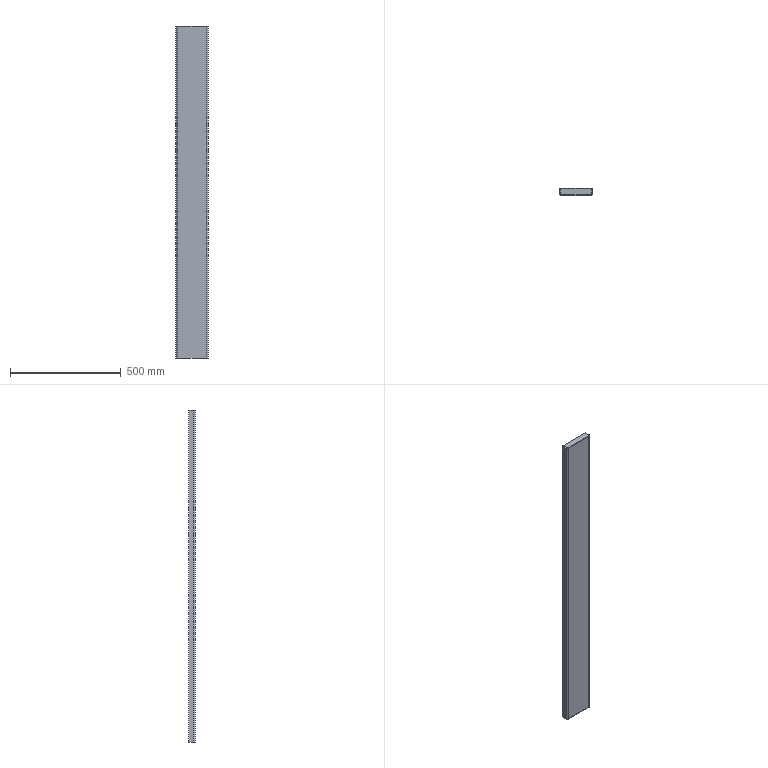Part | SolidWorks | features ICE 2, Extrusion 1 | 3 solids | 30 faces | box 145 x 30 x 1500 mm | volume 892760 mm3 | plane 26 | cylinder 4 | commonest cylinder face diameters 10 x2 16 x2
STEP:
#1=CARTESIAN_POINT('',(145.,-22.,0.));
#2=VERTEX_POINT('',#1);
#3=CARTESIAN_POINT('',(145.,0.,0.));
#4=VERTEX_POINT('',#3);
#5=CARTESIAN_POINT('',(145.,-22.,0.));
#6=DIRECTION('',(0.,1.,0.));
#7=VECTOR('',#6,1000.);
#8=LINE('',#5,#7);
#9=EDGE_CURVE('',#2,#4,#8,.T.);
#10=ORIENTED_EDGE('',*,*,#9,.T.);
#11=CARTESIAN_POINT('',(145.,0.,1500.));
#12=VERTEX_POINT('',#11);
#13=CARTESIAN_POINT('',(145.,0.,1500.));
#14=DIRECTION('',(0.,0.,-1.));
#15=VECTOR('',#14,1000.);
#16=LINE('',#13,#15);
#17=EDGE_CURVE('',#12,#4,#16,.T.);
#18=ORIENTED_EDGE('',*,*,#17,.F.);
#19=CARTESIAN_POINT('',(145.,-22.,1500.));
#20=VERTEX_POINT('',#19);
#21=CARTESIAN_POINT('',(145.,-22.,1500.));
#22=DIRECTION('',(0.,1.,0.));
#23=VECTOR('',#22,1000.);
#24=LINE('',#21,#23);
#25=EDGE_CURVE('',#20,#12,#24,.T.);
#26=ORIENTED_EDGE('',*,*,#25,.F.);
#27=CARTESIAN_POINT('',(145.,-22.,1500.));
#28=DIRECTION('',(0.,0.,-1.));
#29=VECTOR('',#28,1000.);
#30=LINE('',#27,#29);
#31=EDGE_CURVE('',#20,#2,#30,.T.);
#32=ORIENTED_EDGE('',*,*,#31,.T.);
#33=EDGE_LOOP('',(#10,#18,#26,#32));
#34=FACE_OUTER_BOUND('',#33,.T.);
#35=CARTESIAN_POINT('',(145.,-22.,1500.));
#36=DIRECTION('',(-1.,0.,0.));
#37=DIRECTION('',(0.,0.,1.));
#38=AXIS2_PLACEMENT_3D('',#35,#36,#37);
#39=PLANE('',#38);
#40=ADVANCED_FACE('',(#34),#39,.F.);
#41=CARTESIAN_POINT('',(142.,0.,0.));
#42=VERTEX_POINT('',#41);
#43=CARTESIAN_POINT('',(145.,0.,0.));
#44=DIRECTION('',(-1.,0.,0.));
#45=VECTOR('',#44,1000.);
#46=LINE('',#43,#45);
#47=EDGE_CURVE('',#4,#42,#46,.T.);
#48=ORIENTED_EDGE('',*,*,#47,.T.);
#49=CARTESIAN_POINT('',(142.,0.,1500.));
#50=VERTEX_POINT('',#49);
#51=CARTESIAN_POINT('',(142.,0.,1500.));
#52=DIRECTION('',(0.,0.,-1.));
#53=VECTOR('',#52,1000.);
#54=LINE('',#51,#53);
#55=EDGE_CURVE('',#50,#42,#54,.T.);
#56=ORIENTED_EDGE('',*,*,#55,.F.);
#57=CARTESIAN_POINT('',(145.,0.,1500.));
#58=DIRECTION('',(-1.,0.,0.));
#59=VECTOR('',#58,1000.);
#60=LINE('',#57,#59);
#61=EDGE_CURVE('',#12,#50,#60,.T.);
#62=ORIENTED_EDGE('',*,*,#61,.F.);
#63=ORIENTED_EDGE('',*,*,#17,.T.);
#64=EDGE_LOOP('',(#48,#56,#62,#63));
#65=FACE_OUTER_BOUND('',#64,.T.);
#66=CARTESIAN_POINT('',(145.,0.,1500.));
#67=DIRECTION('',(0.,-1.,0.));
#68=DIRECTION('',(0.,0.,-1.));
#69=AXIS2_PLACEMENT_3D('',#66,#67,#68);
#70=PLANE('',#69);
#71=ADVANCED_FACE('',(#65),#70,.F.);
#72=CARTESIAN_POINT('',(142.,-22.,0.));
#73=VERTEX_POINT('',#72);
#74=CARTESIAN_POINT('',(142.,-22.,0.));
#75=DIRECTION('',(0.,1.,0.));
#76=VECTOR('',#75,1000.);
#77=LINE('',#74,#76);
#78=EDGE_CURVE('',#73,#42,#77,.T.);
#79=ORIENTED_EDGE('',*,*,#78,.F.);
#80=CARTESIAN_POINT('',(142.,-22.,1500.));
#81=VERTEX_POINT('',#80);
#82=CARTESIAN_POINT('',(142.,-22.,1500.));
#83=DIRECTION('',(0.,0.,-1.));
#84=VECTOR('',#83,1000.);
#85=LINE('',#82,#84);
#86=EDGE_CURVE('',#81,#73,#85,.T.);
#87=ORIENTED_EDGE('',*,*,#86,.F.);
#88=CARTESIAN_POINT('',(142.,-22.,1500.));
#89=DIRECTION('',(0.,1.,0.));
#90=VECTOR('',#89,1000.);
#91=LINE('',#88,#90);
#92=EDGE_CURVE('',#81,#50,#91,.T.);
#93=ORIENTED_EDGE('',*,*,#92,.T.);
#94=ORIENTED_EDGE('',*,*,#55,.T.);
#95=EDGE_LOOP('',(#79,#87,#93,#94));
#96=FACE_OUTER_BOUND('',#95,.T.);
#97=CARTESIAN_POINT('',(142.,-22.,1500.));
#98=DIRECTION('',(-1.,0.,0.));
#99=DIRECTION('',(0.,0.,1.));
#100=AXIS2_PLACEMENT_3D('',#97,#98,#99);
#101=PLANE('',#100);
#102=ADVANCED_FACE('',(#96),#101,.T.);
#103=CARTESIAN_POINT('',(137.,-27.,0.));
#104=VERTEX_POINT('',#103);
#105=CARTESIAN_POINT('',(137.,-22.,0.));
#106=DIRECTION('',(0.,0.,1.));
#107=DIRECTION('',(1.,0.,0.));
#108=AXIS2_PLACEMENT_3D('',#105,#106,#107);
#109=CIRCLE('',#108,5.);
#110=EDGE_CURVE('',#104,#73,#109,.T.);
#111=ORIENTED_EDGE('',*,*,#110,.F.);
#112=CARTESIAN_POINT('',(137.,-27.,1500.));
#113=VERTEX_POINT('',#112);
#114=CARTESIAN_POINT('',(137.,-27.,1500.));
#115=DIRECTION('',(0.,0.,-1.));
#116=VECTOR('',#115,1000.);
#117=LINE('',#114,#116);
#118=EDGE_CURVE('',#113,#104,#117,.T.);
#119=ORIENTED_EDGE('',*,*,#118,.F.);
#120=CARTESIAN_POINT('',(137.,-22.,1500.));
#121=DIRECTION('',(0.,0.,1.));
#122=DIRECTION('',(1.,0.,0.));
#123=AXIS2_PLACEMENT_3D('',#120,#121,#122);
#124=CIRCLE('',#123,5.);
#125=EDGE_CURVE('',#113,#81,#124,.T.);
#126=ORIENTED_EDGE('',*,*,#125,.T.);
#127=ORIENTED_EDGE('',*,*,#86,.T.);
#128=EDGE_LOOP('',(#111,#119,#126,#127));
#129=FACE_OUTER_BOUND('',#128,.T.);
#130=CARTESIAN_POINT('',(137.,-22.,1500.));
#131=DIRECTION('',(0.,0.,-1.));
#132=DIRECTION('',(-1.,0.,0.));
#133=AXIS2_PLACEMENT_3D('',#130,#131,#132);
#134=CYLINDRICAL_SURFACE('',#133,5.);
#135=ADVANCED_FACE('',(#129),#134,.F.);
#136=CARTESIAN_POINT('',(8.,-27.,0.));
#137=VERTEX_POINT('',#136);
#138=CARTESIAN_POINT('',(8.,-27.,0.));
#139=DIRECTION('',(1.,0.,0.));
#140=VECTOR('',#139,1000.);
#141=LINE('',#138,#140);
#142=EDGE_CURVE('',#137,#104,#141,.T.);
#143=ORIENTED_EDGE('',*,*,#142,.F.);
#144=CARTESIAN_POINT('',(8.,-27.,1500.));
#145=VERTEX_POINT('',#144);
#146=CARTESIAN_POINT('',(8.,-27.,1500.));
#147=DIRECTION('',(0.,0.,-1.));
#148=VECTOR('',#147,1000.);
#149=LINE('',#146,#148);
#150=EDGE_CURVE('',#145,#137,#149,.T.);
#151=ORIENTED_EDGE('',*,*,#150,.F.);
#152=CARTESIAN_POINT('',(8.,-27.,1500.));
#153=DIRECTION('',(1.,0.,0.));
#154=VECTOR('',#153,1000.);
#155=LINE('',#152,#154);
#156=EDGE_CURVE('',#145,#113,#155,.T.);
#157=ORIENTED_EDGE('',*,*,#156,.T.);
#158=ORIENTED_EDGE('',*,*,#118,.T.);
#159=EDGE_LOOP('',(#143,#151,#157,#158));
#160=FACE_OUTER_BOUND('',#159,.T.);
#161=CARTESIAN_POINT('',(8.,-27.,1500.));
#162=DIRECTION('',(0.,1.,0.));
#163=DIRECTION('',(0.,0.,1.));
#164=AXIS2_PLACEMENT_3D('',#161,#162,#163);
#165=PLANE('',#164);
#166=ADVANCED_FACE('',(#160),#165,.T.);
#167=CARTESIAN_POINT('',(3.,-22.,0.));
#168=VERTEX_POINT('',#167);
#169=CARTESIAN_POINT('',(8.,-22.,0.));
#170=DIRECTION('',(0.,0.,1.));
#171=DIRECTION('',(1.,0.,0.));
#172=AXIS2_PLACEMENT_3D('',#169,#170,#171);
#173=CIRCLE('',#172,5.);
#174=EDGE_CURVE('',#168,#137,#173,.T.);
#175=ORIENTED_EDGE('',*,*,#174,.F.);
#176=CARTESIAN_POINT('',(3.,-22.,1500.));
#177=VERTEX_POINT('',#176);
#178=CARTESIAN_POINT('',(3.,-22.,1500.));
#179=DIRECTION('',(0.,0.,-1.));
#180=VECTOR('',#179,1000.);
#181=LINE('',#178,#180);
#182=EDGE_CURVE('',#177,#168,#181,.T.);
#183=ORIENTED_EDGE('',*,*,#182,.F.);
#184=CARTESIAN_POINT('',(8.,-22.,1500.));
#185=DIRECTION('',(0.,0.,1.));
#186=DIRECTION('',(1.,0.,0.));
#187=AXIS2_PLACEMENT_3D('',#184,#185,#186);
#188=CIRCLE('',#187,5.);
#189=EDGE_CURVE('',#177,#145,#188,.T.);
#190=ORIENTED_EDGE('',*,*,#189,.T.);
#191=ORIENTED_EDGE('',*,*,#150,.T.);
#192=EDGE_LOOP('',(#175,#183,#190,#191));
#193=FACE_OUTER_BOUND('',#192,.T.);
#194=CARTESIAN_POINT('',(8.,-22.,1500.));
#195=DIRECTION('',(0.,0.,-1.));
#196=DIRECTION('',(-1.,0.,0.));
#197=AXIS2_PLACEMENT_3D('',#194,#195,#196);
#198=CYLINDRICAL_SURFACE('',#197,5.);
#199=ADVANCED_FACE('',(#193),#198,.F.);
#200=CARTESIAN_POINT('',(3.,0.,0.));
#201=VERTEX_POINT('',#200);
#202=CARTESIAN_POINT('',(3.,0.,0.));
#203=DIRECTION('',(0.,-1.,0.));
#204=VECTOR('',#203,1000.);
#205=LINE('',#202,#204);
#206=EDGE_CURVE('',#201,#168,#205,.T.);
#207=ORIENTED_EDGE('',*,*,#206,.F.);
#208=CARTESIAN_POINT('',(3.,0.,1500.));
#209=VERTEX_POINT('',#208);
#210=CARTESIAN_POINT('',(3.,0.,1500.));
#211=DIRECTION('',(0.,0.,-1.));
#212=VECTOR('',#211,1000.);
#213=LINE('',#210,#212);
#214=EDGE_CURVE('',#209,#201,#213,.T.);
#215=ORIENTED_EDGE('',*,*,#214,.F.);
#216=CARTESIAN_POINT('',(3.,0.,1500.));
#217=DIRECTION('',(0.,-1.,0.));
#218=VECTOR('',#217,1000.);
#219=LINE('',#216,#218);
#220=EDGE_CURVE('',#209,#177,#219,.T.);
#221=ORIENTED_EDGE('',*,*,#220,.T.);
#222=ORIENTED_EDGE('',*,*,#182,.T.);
#223=EDGE_LOOP('',(#207,#215,#221,#222));
#224=FACE_OUTER_BOUND('',#223,.T.);
#225=CARTESIAN_POINT('',(3.,0.,1500.));
#226=DIRECTION('',(1.,0.,0.));
#227=DIRECTION('',(0.,0.,-1.));
#228=AXIS2_PLACEMENT_3D('',#225,#226,#227);
#229=PLANE('',#228);
#230=ADVANCED_FACE('',(#224),#229,.T.);
#231=CARTESIAN_POINT('',(0.,0.,0.));
#232=VERTEX_POINT('',#231);
#233=CARTESIAN_POINT('',(0.,0.,0.));
#234=DIRECTION('',(1.,0.,0.));
#235=VECTOR('',#234,1000.);
#236=LINE('',#233,#235);
#237=EDGE_CURVE('',#232,#201,#236,.T.);
#238=ORIENTED_EDGE('',*,*,#237,.F.);
#239=CARTESIAN_POINT('',(0.,0.,1500.));
#240=VERTEX_POINT('',#239);
#241=CARTESIAN_POINT('',(0.,0.,1500.));
#242=DIRECTION('',(0.,0.,-1.));
#243=VECTOR('',#242,1000.);
#244=LINE('',#241,#243);
#245=EDGE_CURVE('',#240,#232,#244,.T.);
#246=ORIENTED_EDGE('',*,*,#245,.F.);
#247=CARTESIAN_POINT('',(0.,0.,1500.));
#248=DIRECTION('',(1.,0.,0.));
#249=VECTOR('',#248,1000.);
#250=LINE('',#247,#249);
#251=EDGE_CURVE('',#240,#209,#250,.T.);
#252=ORIENTED_EDGE('',*,*,#251,.T.);
#253=ORIENTED_EDGE('',*,*,#214,.T.);
#254=EDGE_LOOP('',(#238,#246,#252,#253));
#255=FACE_OUTER_BOUND('',#254,.T.);
#256=CARTESIAN_POINT('',(0.,0.,1500.));
#257=DIRECTION('',(0.,1.,0.));
#258=DIRECTION('',(0.,0.,1.));
#259=AXIS2_PLACEMENT_3D('',#256,#257,#258);
#260=PLANE('',#259);
#261=ADVANCED_FACE('',(#255),#260,.T.);
#262=CARTESIAN_POINT('',(0.,-22.,0.));
#263=VERTEX_POINT('',#262);
#264=CARTESIAN_POINT('',(0.,0.,0.));
#265=DIRECTION('',(0.,-1.,0.));
#266=VECTOR('',#265,1000.);
#267=LINE('',#264,#266);
#268=EDGE_CURVE('',#232,#263,#267,.T.);
#269=ORIENTED_EDGE('',*,*,#268,.T.);
#270=CARTESIAN_POINT('',(0.,-22.,1500.));
#271=VERTEX_POINT('',#270);
#272=CARTESIAN_POINT('',(0.,-22.,1500.));
#273=DIRECTION('',(0.,0.,-1.));
#274=VECTOR('',#273,1000.);
#275=LINE('',#272,#274);
#276=EDGE_CURVE('',#271,#263,#275,.T.);
#277=ORIENTED_EDGE('',*,*,#276,.F.);
#278=CARTESIAN_POINT('',(0.,0.,1500.));
#279=DIRECTION('',(0.,-1.,0.));
#280=VECTOR('',#279,1000.);
#281=LINE('',#278,#280);
#282=EDGE_CURVE('',#240,#271,#281,.T.);
#283=ORIENTED_EDGE('',*,*,#282,.F.);
#284=ORIENTED_EDGE('',*,*,#245,.T.);
#285=EDGE_LOOP('',(#269,#277,#283,#284));
#286=FACE_OUTER_BOUND('',#285,.T.);
#287=CARTESIAN_POINT('',(0.,0.,1500.));
#288=DIRECTION('',(1.,0.,0.));
#289=DIRECTION('',(0.,0.,-1.));
#290=AXIS2_PLACEMENT_3D('',#287,#288,#289);
#291=PLANE('',#290);
#292=ADVANCED_FACE('',(#286),#291,.F.);
#293=CARTESIAN_POINT('',(8.,-30.,0.));
#294=VERTEX_POINT('',#293);
#295=CARTESIAN_POINT('',(8.,-22.,0.));
#296=DIRECTION('',(0.,0.,1.));
#297=DIRECTION('',(1.,0.,0.));
#298=AXIS2_PLACEMENT_3D('',#295,#296,#297);
#299=CIRCLE('',#298,8.);
#300=EDGE_CURVE('',#263,#294,#299,.T.);
#301=ORIENTED_EDGE('',*,*,#300,.T.);
#302=CARTESIAN_POINT('',(8.,-30.,1500.));
#303=VERTEX_POINT('',#302);
#304=CARTESIAN_POINT('',(8.,-30.,1500.));
#305=DIRECTION('',(0.,0.,-1.));
#306=VECTOR('',#305,1000.);
#307=LINE('',#304,#306);
#308=EDGE_CURVE('',#303,#294,#307,.T.);
#309=ORIENTED_EDGE('',*,*,#308,.F.);
#310=CARTESIAN_POINT('',(8.,-22.,1500.));
#311=DIRECTION('',(0.,0.,1.));
#312=DIRECTION('',(1.,0.,0.));
#313=AXIS2_PLACEMENT_3D('',#310,#311,#312);
#314=CIRCLE('',#313,8.);
#315=EDGE_CURVE('',#271,#303,#314,.T.);
#316=ORIENTED_EDGE('',*,*,#315,.F.);
#317=ORIENTED_EDGE('',*,*,#276,.T.);
#318=EDGE_LOOP('',(#301,#309,#316,#317));
#319=FACE_OUTER_BOUND('',#318,.T.);
#320=CARTESIAN_POINT('',(8.,-22.,1500.));
#321=DIRECTION('',(0.,0.,-1.));
#322=DIRECTION('',(-1.,0.,0.));
#323=AXIS2_PLACEMENT_3D('',#320,#321,#322);
#324=CYLINDRICAL_SURFACE('',#323,8.);
#325=ADVANCED_FACE('',(#319),#324,.T.);
#326=CARTESIAN_POINT('',(137.,-30.,0.));
#327=VERTEX_POINT('',#326);
#328=CARTESIAN_POINT('',(8.,-30.,0.));
#329=DIRECTION('',(1.,0.,0.));
#330=VECTOR('',#329,1000.);
#331=LINE('',#328,#330);
#332=EDGE_CURVE('',#294,#327,#331,.T.);
#333=ORIENTED_EDGE('',*,*,#332,.T.);
#334=CARTESIAN_POINT('',(137.,-30.,1500.));
#335=VERTEX_POINT('',#334);
#336=CARTESIAN_POINT('',(137.,-30.,1500.));
#337=DIRECTION('',(0.,0.,-1.));
#338=VECTOR('',#337,1000.);
#339=LINE('',#336,#338);
#340=EDGE_CURVE('',#335,#327,#339,.T.);
#341=ORIENTED_EDGE('',*,*,#340,.F.);
#342=CARTESIAN_POINT('',(8.,-30.,1500.));
#343=DIRECTION('',(1.,0.,0.));
#344=VECTOR('',#343,1000.);
#345=LINE('',#342,#344);
#346=EDGE_CURVE('',#303,#335,#345,.T.);
#347=ORIENTED_EDGE('',*,*,#346,.F.);
#348=ORIENTED_EDGE('',*,*,#308,.T.);
#349=EDGE_LOOP('',(#333,#341,#347,#348));
#350=FACE_OUTER_BOUND('',#349,.T.);
#351=CARTESIAN_POINT('',(8.,-30.,1500.));
#352=DIRECTION('',(0.,1.,0.));
#353=DIRECTION('',(0.,0.,1.));
#354=AXIS2_PLACEMENT_3D('',#351,#352,#353);
#355=PLANE('',#354);
#356=ADVANCED_FACE('',(#350),#355,.F.);
#357=CARTESIAN_POINT('',(137.,-22.,0.));
#358=DIRECTION('',(0.,0.,1.));
#359=DIRECTION('',(1.,0.,0.));
#360=AXIS2_PLACEMENT_3D('',#357,#358,#359);
#361=CIRCLE('',#360,8.);
#362=EDGE_CURVE('',#327,#2,#361,.T.);
#363=ORIENTED_EDGE('',*,*,#362,.T.);
#364=ORIENTED_EDGE('',*,*,#31,.F.);
#365=CARTESIAN_POINT('',(137.,-22.,1500.));
#366=DIRECTION('',(0.,0.,1.));
#367=DIRECTION('',(1.,0.,0.));
#368=AXIS2_PLACEMENT_3D('',#365,#366,#367);
#369=CIRCLE('',#368,8.);
#370=EDGE_CURVE('',#335,#20,#369,.T.);
#371=ORIENTED_EDGE('',*,*,#370,.F.);
#372=ORIENTED_EDGE('',*,*,#340,.T.);
#373=EDGE_LOOP('',(#363,#364,#371,#372));
#374=FACE_OUTER_BOUND('',#373,.T.);
#375=CARTESIAN_POINT('',(137.,-22.,1500.));
#376=DIRECTION('',(0.,0.,-1.));
#377=DIRECTION('',(-1.,0.,0.));
#378=AXIS2_PLACEMENT_3D('',#375,#376,#377);
#379=CYLINDRICAL_SURFACE('',#378,8.);
#380=ADVANCED_FACE('',(#374),#379,.T.);
#381=ORIENTED_EDGE('',*,*,#25,.T.);
#382=ORIENTED_EDGE('',*,*,#61,.T.);
#383=ORIENTED_EDGE('',*,*,#92,.F.);
#384=ORIENTED_EDGE('',*,*,#125,.F.);
#385=ORIENTED_EDGE('',*,*,#156,.F.);
#386=ORIENTED_EDGE('',*,*,#189,.F.);
#387=ORIENTED_EDGE('',*,*,#220,.F.);
#388=ORIENTED_EDGE('',*,*,#251,.F.);
#389=ORIENTED_EDGE('',*,*,#282,.T.);
#390=ORIENTED_EDGE('',*,*,#315,.T.);
#391=ORIENTED_EDGE('',*,*,#346,.T.);
#392=ORIENTED_EDGE('',*,*,#370,.T.);
#393=EDGE_LOOP('',(#381,#382,#383,#384,#385,#386,#387,#388,#389,#390,#391,#392));
#394=FACE_OUTER_BOUND('',#393,.T.);
#395=CARTESIAN_POINT('',(137.,-22.,1500.));
#396=DIRECTION('',(0.,0.,1.));
#397=DIRECTION('',(1.,0.,0.));
#398=AXIS2_PLACEMENT_3D('',#395,#396,#397);
#399=PLANE('',#398);
#400=ADVANCED_FACE('',(#394),#399,.T.);
#401=ORIENTED_EDGE('',*,*,#9,.F.);
#402=ORIENTED_EDGE('',*,*,#362,.F.);
#403=ORIENTED_EDGE('',*,*,#332,.F.);
#404=ORIENTED_EDGE('',*,*,#300,.F.);
#405=ORIENTED_EDGE('',*,*,#268,.F.);
#406=ORIENTED_EDGE('',*,*,#237,.T.);
#407=ORIENTED_EDGE('',*,*,#206,.T.);
#408=ORIENTED_EDGE('',*,*,#174,.T.);
#409=ORIENTED_EDGE('',*,*,#142,.T.);
#410=ORIENTED_EDGE('',*,*,#110,.T.);
#411=ORIENTED_EDGE('',*,*,#78,.T.);
#412=ORIENTED_EDGE('',*,*,#47,.F.);
#413=EDGE_LOOP('',(#401,#402,#403,#404,#405,#406,#407,#408,#409,#410,#411,#412));
#414=FACE_OUTER_BOUND('',#413,.T.);
#415=CARTESIAN_POINT('',(137.,-22.,0.));
#416=DIRECTION('',(0.,0.,1.));
#417=DIRECTION('',(1.,0.,0.));
#418=AXIS2_PLACEMENT_3D('',#415,#416,#417);
#419=PLANE('',#418);
#420=ADVANCED_FACE('',(#414),#419,.F.);
#421=CLOSED_SHELL('',(#40,#71,#102,#135,#166,#199,#230,#261,#292,#325,#356,#380,#400,#420));
#422=MANIFOLD_SOLID_BREP('',#421);
#423=CARTESIAN_POINT('',(8.,-27.,1500.));
#424=VERTEX_POINT('',#423);
#425=CARTESIAN_POINT('',(3.,-22.,1500.));
#426=VERTEX_POINT('',#425);
#427=CARTESIAN_POINT('',(8.,-27.,1500.));
#428=DIRECTION('',(-0.7071,0.7071,0.));
#429=VECTOR('',#428,1000.);
#430=LINE('',#427,#429);
#431=EDGE_CURVE('',#424,#426,#430,.T.);
#432=ORIENTED_EDGE('',*,*,#431,.T.);
#433=CARTESIAN_POINT('',(3.,-22.,1497.));
#434=VERTEX_POINT('',#433);
#435=CARTESIAN_POINT('',(3.,-22.,1497.));
#436=DIRECTION('',(0.,0.,1.));
#437=VECTOR('',#436,1000.);
#438=LINE('',#435,#437);
#439=EDGE_CURVE('',#434,#426,#438,.T.);
#440=ORIENTED_EDGE('',*,*,#439,.F.);
#441=CARTESIAN_POINT('',(8.,-27.,1497.));
#442=VERTEX_POINT('',#441);
#443=CARTESIAN_POINT('',(8.,-27.,1497.));
#444=DIRECTION('',(-0.7071,0.7071,0.));
#445=VECTOR('',#444,1000.);
#446=LINE('',#443,#445);
#447=EDGE_CURVE('',#442,#434,#446,.T.);
#448=ORIENTED_EDGE('',*,*,#447,.F.);
#449=CARTESIAN_POINT('',(8.,-27.,1497.));
#450=DIRECTION('',(0.,0.,1.));
#451=VECTOR('',#450,1000.);
#452=LINE('',#449,#451);
#453=EDGE_CURVE('',#442,#424,#452,.T.);
#454=ORIENTED_EDGE('',*,*,#453,.T.);
#455=EDGE_LOOP('',(#432,#440,#448,#454));
#456=FACE_OUTER_BOUND('',#455,.T.);
#457=CARTESIAN_POINT('',(8.,-27.,1497.));
#458=DIRECTION('',(0.7071,0.7071,0.));
#459=DIRECTION('',(-0.7071,0.7071,0.));
#460=AXIS2_PLACEMENT_3D('',#457,#458,#459);
#461=PLANE('',#460);
#462=ADVANCED_FACE('',(#456),#461,.F.);
#463=CARTESIAN_POINT('',(3.,0.,1500.));
#464=VERTEX_POINT('',#463);
#465=CARTESIAN_POINT('',(3.,-22.,1500.));
#466=DIRECTION('',(0.,1.,0.));
#467=VECTOR('',#466,1000.);
#468=LINE('',#465,#467);
#469=EDGE_CURVE('',#426,#464,#468,.T.);
#470=ORIENTED_EDGE('',*,*,#469,.T.);
#471=CARTESIAN_POINT('',(3.,0.,1497.));
#472=VERTEX_POINT('',#471);
#473=CARTESIAN_POINT('',(3.,0.,1497.));
#474=DIRECTION('',(0.,0.,1.));
#475=VECTOR('',#474,1000.);
#476=LINE('',#473,#475);
#477=EDGE_CURVE('',#472,#464,#476,.T.);
#478=ORIENTED_EDGE('',*,*,#477,.F.);
#479=CARTESIAN_POINT('',(3.,-22.,1497.));
#480=DIRECTION('',(0.,1.,0.));
#481=VECTOR('',#480,1000.);
#482=LINE('',#479,#481);
#483=EDGE_CURVE('',#434,#472,#482,.T.);
#484=ORIENTED_EDGE('',*,*,#483,.F.);
#485=ORIENTED_EDGE('',*,*,#439,.T.);
#486=EDGE_LOOP('',(#470,#478,#484,#485));
#487=FACE_OUTER_BOUND('',#486,.T.);
#488=CARTESIAN_POINT('',(3.,-22.,1497.));
#489=DIRECTION('',(1.,0.,0.));
#490=DIRECTION('',(0.,1.,0.));
#491=AXIS2_PLACEMENT_3D('',#488,#489,#490);
#492=PLANE('',#491);
#493=ADVANCED_FACE('',(#487),#492,.F.);
#494=CARTESIAN_POINT('',(142.,0.,1500.));
#495=VERTEX_POINT('',#494);
#496=CARTESIAN_POINT('',(3.,0.,1500.));
#497=DIRECTION('',(1.,0.,0.));
#498=VECTOR('',#497,1000.);
#499=LINE('',#496,#498);
#500=EDGE_CURVE('',#464,#495,#499,.T.);
#501=ORIENTED_EDGE('',*,*,#500,.T.);
#502=CARTESIAN_POINT('',(142.,0.,1497.));
#503=VERTEX_POINT('',#502);
#504=CARTESIAN_POINT('',(142.,0.,1497.));
#505=DIRECTION('',(0.,0.,1.));
#506=VECTOR('',#505,1000.);
#507=LINE('',#504,#506);
#508=EDGE_CURVE('',#503,#495,#507,.T.);
#509=ORIENTED_EDGE('',*,*,#508,.F.);
#510=CARTESIAN_POINT('',(3.,0.,1497.));
#511=DIRECTION('',(1.,0.,0.));
#512=VECTOR('',#511,1000.);
#513=LINE('',#510,#512);
#514=EDGE_CURVE('',#472,#503,#513,.T.);
#515=ORIENTED_EDGE('',*,*,#514,.F.);
#516=ORIENTED_EDGE('',*,*,#477,.T.);
#517=EDGE_LOOP('',(#501,#509,#515,#516));
#518=FACE_OUTER_BOUND('',#517,.T.);
#519=CARTESIAN_POINT('',(3.,0.,1497.));
#520=DIRECTION('',(0.,-1.,0.));
#521=DIRECTION('',(0.,0.,-1.));
#522=AXIS2_PLACEMENT_3D('',#519,#520,#521);
#523=PLANE('',#522);
#524=ADVANCED_FACE('',(#518),#523,.F.);
#525=CARTESIAN_POINT('',(142.,-22.,1500.));
#526=VERTEX_POINT('',#525);
#527=CARTESIAN_POINT('',(142.,0.,1500.));
#528=DIRECTION('',(0.,-1.,0.));
#529=VECTOR('',#528,1000.);
#530=LINE('',#527,#529);
#531=EDGE_CURVE('',#495,#526,#530,.T.);
#532=ORIENTED_EDGE('',*,*,#531,.T.);
#533=CARTESIAN_POINT('',(142.,-22.,1497.));
#534=VERTEX_POINT('',#533);
#535=CARTESIAN_POINT('',(142.,-22.,1497.));
#536=DIRECTION('',(0.,0.,1.));
#537=VECTOR('',#536,1000.);
#538=LINE('',#535,#537);
#539=EDGE_CURVE('',#534,#526,#538,.T.);
#540=ORIENTED_EDGE('',*,*,#539,.F.);
#541=CARTESIAN_POINT('',(142.,0.,1497.));
#542=DIRECTION('',(0.,-1.,0.));
#543=VECTOR('',#542,1000.);
#544=LINE('',#541,#543);
#545=EDGE_CURVE('',#503,#534,#544,.T.);
#546=ORIENTED_EDGE('',*,*,#545,.F.);
#547=ORIENTED_EDGE('',*,*,#508,.T.);
#548=EDGE_LOOP('',(#532,#540,#546,#547));
#549=FACE_OUTER_BOUND('',#548,.T.);
#550=CARTESIAN_POINT('',(142.,0.,1497.));
#551=DIRECTION('',(-1.,0.,0.));
#552=DIRECTION('',(0.,0.,1.));
#553=AXIS2_PLACEMENT_3D('',#550,#551,#552);
#554=PLANE('',#553);
#555=ADVANCED_FACE('',(#549),#554,.F.);
#556=CARTESIAN_POINT('',(137.,-27.,1500.));
#557=VERTEX_POINT('',#556);
#558=CARTESIAN_POINT('',(142.,-22.,1500.));
#559=DIRECTION('',(-0.7071,-0.7071,0.));
#560=VECTOR('',#559,1000.);
#561=LINE('',#558,#560);
#562=EDGE_CURVE('',#526,#557,#561,.T.);
#563=ORIENTED_EDGE('',*,*,#562,.T.);
#564=CARTESIAN_POINT('',(137.,-27.,1497.));
#565=VERTEX_POINT('',#564);
#566=CARTESIAN_POINT('',(137.,-27.,1497.));
#567=DIRECTION('',(0.,0.,1.));
#568=VECTOR('',#567,1000.);
#569=LINE('',#566,#568);
#570=EDGE_CURVE('',#565,#557,#569,.T.);
#571=ORIENTED_EDGE('',*,*,#570,.F.);
#572=CARTESIAN_POINT('',(142.,-22.,1497.));
#573=DIRECTION('',(-0.7071,-0.7071,0.));
#574=VECTOR('',#573,1000.);
#575=LINE('',#572,#574);
#576=EDGE_CURVE('',#534,#565,#575,.T.);
#577=ORIENTED_EDGE('',*,*,#576,.F.);
#578=ORIENTED_EDGE('',*,*,#539,.T.);
#579=EDGE_LOOP('',(#563,#571,#577,#578));
#580=FACE_OUTER_BOUND('',#579,.T.);
#581=CARTESIAN_POINT('',(142.,-22.,1497.));
#582=DIRECTION('',(-0.7071,0.7071,0.));
#583=DIRECTION('',(-0.7071,-0.7071,0.));
#584=AXIS2_PLACEMENT_3D('',#581,#582,#583);
#585=PLANE('',#584);
#586=ADVANCED_FACE('',(#580),#585,.F.);
#587=CARTESIAN_POINT('',(137.,-27.,1500.));
#588=DIRECTION('',(-1.,0.,0.));
#589=VECTOR('',#588,1000.);
#590=LINE('',#587,#589);
#591=EDGE_CURVE('',#557,#424,#590,.T.);
#592=ORIENTED_EDGE('',*,*,#591,.T.);
#593=ORIENTED_EDGE('',*,*,#453,.F.);
#594=CARTESIAN_POINT('',(137.,-27.,1497.));
#595=DIRECTION('',(-1.,0.,0.));
#596=VECTOR('',#595,1000.);
#597=LINE('',#594,#596);
#598=EDGE_CURVE('',#565,#442,#597,.T.);
#599=ORIENTED_EDGE('',*,*,#598,.F.);
#600=ORIENTED_EDGE('',*,*,#570,.T.);
#601=EDGE_LOOP('',(#592,#593,#599,#600));
#602=FACE_OUTER_BOUND('',#601,.T.);
#603=CARTESIAN_POINT('',(137.,-27.,1497.));
#604=DIRECTION('',(0.,1.,0.));
#605=DIRECTION('',(0.,0.,1.));
#606=AXIS2_PLACEMENT_3D('',#603,#604,#605);
#607=PLANE('',#606);
#608=ADVANCED_FACE('',(#602),#607,.F.);
#609=ORIENTED_EDGE('',*,*,#447,.T.);
#610=ORIENTED_EDGE('',*,*,#483,.T.);
#611=ORIENTED_EDGE('',*,*,#514,.T.);
#612=ORIENTED_EDGE('',*,*,#545,.T.);
#613=ORIENTED_EDGE('',*,*,#576,.T.);
#614=ORIENTED_EDGE('',*,*,#598,.T.);
#615=EDGE_LOOP('',(#609,#610,#611,#612,#613,#614));
#616=FACE_OUTER_BOUND('',#615,.T.);
#617=CARTESIAN_POINT('',(0.,0.,1497.));
#618=DIRECTION('',(0.,0.,1.));
#619=DIRECTION('',(1.,0.,0.));
#620=AXIS2_PLACEMENT_3D('',#617,#618,#619);
#621=PLANE('',#620);
#622=ADVANCED_FACE('',(#616),#621,.F.);
#623=ORIENTED_EDGE('',*,*,#431,.F.);
#624=ORIENTED_EDGE('',*,*,#591,.F.);
#625=ORIENTED_EDGE('',*,*,#562,.F.);
#626=ORIENTED_EDGE('',*,*,#531,.F.);
#627=ORIENTED_EDGE('',*,*,#500,.F.);
#628=ORIENTED_EDGE('',*,*,#469,.F.);
#629=EDGE_LOOP('',(#623,#624,#625,#626,#627,#628));
#630=FACE_OUTER_BOUND('',#629,.T.);
#631=CARTESIAN_POINT('',(0.,0.,1500.));
#632=DIRECTION('',(0.,0.,1.));
#633=DIRECTION('',(1.,0.,0.));
#634=AXIS2_PLACEMENT_3D('',#631,#632,#633);
#635=PLANE('',#634);
#636=ADVANCED_FACE('',(#630),#635,.T.);
#637=CLOSED_SHELL('',(#462,#493,#524,#555,#586,#608,#622,#636));
#638=MANIFOLD_SOLID_BREP('',#637);
#639=CARTESIAN_POINT('',(142.,0.,0.));
#640=VERTEX_POINT('',#639);
#641=CARTESIAN_POINT('',(142.,-22.,0.));
#642=VERTEX_POINT('',#641);
#643=CARTESIAN_POINT('',(142.,-22.,0.));
#644=DIRECTION('',(0.,-1.,0.));
#645=VECTOR('',#644,1000.);
#646=LINE('',#643,#645);
#647=EDGE_CURVE('',#640,#642,#646,.T.);
#648=ORIENTED_EDGE('',*,*,#647,.F.);
#649=CARTESIAN_POINT('',(142.,0.,3.));
#650=VERTEX_POINT('',#649);
#651=CARTESIAN_POINT('',(142.,0.,3.));
#652=DIRECTION('',(0.,0.,-1.));
#653=VECTOR('',#652,1000.);
#654=LINE('',#651,#653);
#655=EDGE_CURVE('',#650,#640,#654,.T.);
#656=ORIENTED_EDGE('',*,*,#655,.F.);
#657=CARTESIAN_POINT('',(142.,-22.,3.));
#658=VERTEX_POINT('',#657);
#659=CARTESIAN_POINT('',(142.,-22.,3.));
#660=DIRECTION('',(0.,-1.,0.));
#661=VECTOR('',#660,1000.);
#662=LINE('',#659,#661);
#663=EDGE_CURVE('',#650,#658,#662,.T.);
#664=ORIENTED_EDGE('',*,*,#663,.T.);
#665=CARTESIAN_POINT('',(142.,-22.,3.));
#666=DIRECTION('',(0.,0.,-1.));
#667=VECTOR('',#666,1000.);
#668=LINE('',#665,#667);
#669=EDGE_CURVE('',#658,#642,#668,.T.);
#670=ORIENTED_EDGE('',*,*,#669,.T.);
#671=EDGE_LOOP('',(#648,#656,#664,#670));
#672=FACE_OUTER_BOUND('',#671,.T.);
#673=CARTESIAN_POINT('',(142.,-22.,3.));
#674=DIRECTION('',(1.,0.,0.));
#675=DIRECTION('',(0.,0.,-1.));
#676=AXIS2_PLACEMENT_3D('',#673,#674,#675);
#677=PLANE('',#676);
#678=ADVANCED_FACE('',(#672),#677,.T.);
#679=CARTESIAN_POINT('',(3.,0.,0.));
#680=VERTEX_POINT('',#679);
#681=CARTESIAN_POINT('',(142.,0.,0.));
#682=DIRECTION('',(1.,0.,0.));
#683=VECTOR('',#682,1000.);
#684=LINE('',#681,#683);
#685=EDGE_CURVE('',#680,#640,#684,.T.);
#686=ORIENTED_EDGE('',*,*,#685,.F.);
#687=CARTESIAN_POINT('',(3.,0.,3.));
#688=VERTEX_POINT('',#687);
#689=CARTESIAN_POINT('',(3.,0.,3.));
#690=DIRECTION('',(0.,0.,-1.));
#691=VECTOR('',#690,1000.);
#692=LINE('',#689,#691);
#693=EDGE_CURVE('',#688,#680,#692,.T.);
#694=ORIENTED_EDGE('',*,*,#693,.F.);
#695=CARTESIAN_POINT('',(142.,0.,3.));
#696=DIRECTION('',(1.,0.,0.));
#697=VECTOR('',#696,1000.);
#698=LINE('',#695,#697);
#699=EDGE_CURVE('',#688,#650,#698,.T.);
#700=ORIENTED_EDGE('',*,*,#699,.T.);
#701=ORIENTED_EDGE('',*,*,#655,.T.);
#702=EDGE_LOOP('',(#686,#694,#700,#701));
#703=FACE_OUTER_BOUND('',#702,.T.);
#704=CARTESIAN_POINT('',(142.,0.,3.));
#705=DIRECTION('',(0.,1.,0.));
#706=DIRECTION('',(0.,0.,1.));
#707=AXIS2_PLACEMENT_3D('',#704,#705,#706);
#708=PLANE('',#707);
#709=ADVANCED_FACE('',(#703),#708,.T.);
#710=CARTESIAN_POINT('',(3.,-22.,0.));
#711=VERTEX_POINT('',#710);
#712=CARTESIAN_POINT('',(3.,0.,0.));
#713=DIRECTION('',(0.,1.,0.));
#714=VECTOR('',#713,1000.);
#715=LINE('',#712,#714);
#716=EDGE_CURVE('',#711,#680,#715,.T.);
#717=ORIENTED_EDGE('',*,*,#716,.F.);
#718=CARTESIAN_POINT('',(3.,-22.,3.));
#719=VERTEX_POINT('',#718);
#720=CARTESIAN_POINT('',(3.,-22.,3.));
#721=DIRECTION('',(0.,0.,-1.));
#722=VECTOR('',#721,1000.);
#723=LINE('',#720,#722);
#724=EDGE_CURVE('',#719,#711,#723,.T.);
#725=ORIENTED_EDGE('',*,*,#724,.F.);
#726=CARTESIAN_POINT('',(3.,0.,3.));
#727=DIRECTION('',(0.,1.,0.));
#728=VECTOR('',#727,1000.);
#729=LINE('',#726,#728);
#730=EDGE_CURVE('',#719,#688,#729,.T.);
#731=ORIENTED_EDGE('',*,*,#730,.T.);
#732=ORIENTED_EDGE('',*,*,#693,.T.);
#733=EDGE_LOOP('',(#717,#725,#731,#732));
#734=FACE_OUTER_BOUND('',#733,.T.);
#735=CARTESIAN_POINT('',(3.,0.,3.));
#736=DIRECTION('',(-1.,0.,0.));
#737=DIRECTION('',(0.,0.,1.));
#738=AXIS2_PLACEMENT_3D('',#735,#736,#737);
#739=PLANE('',#738);
#740=ADVANCED_FACE('',(#734),#739,.T.);
#741=CARTESIAN_POINT('',(8.,-27.,0.));
#742=VERTEX_POINT('',#741);
#743=CARTESIAN_POINT('',(3.,-22.,0.));
#744=DIRECTION('',(-0.7071,0.7071,0.));
#745=VECTOR('',#744,1000.);
#746=LINE('',#743,#745);
#747=EDGE_CURVE('',#742,#711,#746,.T.);
#748=ORIENTED_EDGE('',*,*,#747,.F.);
#749=CARTESIAN_POINT('',(8.,-27.,3.));
#750=VERTEX_POINT('',#749);
#751=CARTESIAN_POINT('',(8.,-27.,3.));
#752=DIRECTION('',(0.,0.,-1.));
#753=VECTOR('',#752,1000.);
#754=LINE('',#751,#753);
#755=EDGE_CURVE('',#750,#742,#754,.T.);
#756=ORIENTED_EDGE('',*,*,#755,.F.);
#757=CARTESIAN_POINT('',(3.,-22.,3.));
#758=DIRECTION('',(-0.7071,0.7071,0.));
#759=VECTOR('',#758,1000.);
#760=LINE('',#757,#759);
#761=EDGE_CURVE('',#750,#719,#760,.T.);
#762=ORIENTED_EDGE('',*,*,#761,.T.);
#763=ORIENTED_EDGE('',*,*,#724,.T.);
#764=EDGE_LOOP('',(#748,#756,#762,#763));
#765=FACE_OUTER_BOUND('',#764,.T.);
#766=CARTESIAN_POINT('',(3.,-22.,3.));
#767=DIRECTION('',(-0.7071,-0.7071,0.));
#768=DIRECTION('',(0.7071,-0.7071,0.));
#769=AXIS2_PLACEMENT_3D('',#766,#767,#768);
#770=PLANE('',#769);
#771=ADVANCED_FACE('',(#765),#770,.T.);
#772=CARTESIAN_POINT('',(137.,-27.,0.));
#773=VERTEX_POINT('',#772);
#774=CARTESIAN_POINT('',(8.,-27.,0.));
#775=DIRECTION('',(-1.,0.,0.));
#776=VECTOR('',#775,1000.);
#777=LINE('',#774,#776);
#778=EDGE_CURVE('',#773,#742,#777,.T.);
#779=ORIENTED_EDGE('',*,*,#778,.F.);
#780=CARTESIAN_POINT('',(137.,-27.,3.));
#781=VERTEX_POINT('',#780);
#782=CARTESIAN_POINT('',(137.,-27.,3.));
#783=DIRECTION('',(0.,0.,-1.));
#784=VECTOR('',#783,1000.);
#785=LINE('',#782,#784);
#786=EDGE_CURVE('',#781,#773,#785,.T.);
#787=ORIENTED_EDGE('',*,*,#786,.F.);
#788=CARTESIAN_POINT('',(8.,-27.,3.));
#789=DIRECTION('',(-1.,0.,0.));
#790=VECTOR('',#789,1000.);
#791=LINE('',#788,#790);
#792=EDGE_CURVE('',#781,#750,#791,.T.);
#793=ORIENTED_EDGE('',*,*,#792,.T.);
#794=ORIENTED_EDGE('',*,*,#755,.T.);
#795=EDGE_LOOP('',(#779,#787,#793,#794));
#796=FACE_OUTER_BOUND('',#795,.T.);
#797=CARTESIAN_POINT('',(8.,-27.,3.));
#798=DIRECTION('',(0.,-1.,0.));
#799=DIRECTION('',(0.,0.,-1.));
#800=AXIS2_PLACEMENT_3D('',#797,#798,#799);
#801=PLANE('',#800);
#802=ADVANCED_FACE('',(#796),#801,.T.);
#803=CARTESIAN_POINT('',(137.,-27.,0.));
#804=DIRECTION('',(-0.7071,-0.7071,0.));
#805=VECTOR('',#804,1000.);
#806=LINE('',#803,#805);
#807=EDGE_CURVE('',#642,#773,#806,.T.);
#808=ORIENTED_EDGE('',*,*,#807,.F.);
#809=ORIENTED_EDGE('',*,*,#669,.F.);
#810=CARTESIAN_POINT('',(137.,-27.,3.));
#811=DIRECTION('',(-0.7071,-0.7071,0.));
#812=VECTOR('',#811,1000.);
#813=LINE('',#810,#812);
#814=EDGE_CURVE('',#658,#781,#813,.T.);
#815=ORIENTED_EDGE('',*,*,#814,.T.);
#816=ORIENTED_EDGE('',*,*,#786,.T.);
#817=EDGE_LOOP('',(#808,#809,#815,#816));
#818=FACE_OUTER_BOUND('',#817,.T.);
#819=CARTESIAN_POINT('',(137.,-27.,3.));
#820=DIRECTION('',(0.7071,-0.7071,0.));
#821=DIRECTION('',(0.7071,0.7071,0.));
#822=AXIS2_PLACEMENT_3D('',#819,#820,#821);
#823=PLANE('',#822);
#824=ADVANCED_FACE('',(#818),#823,.T.);
#825=ORIENTED_EDGE('',*,*,#663,.F.);
#826=ORIENTED_EDGE('',*,*,#699,.F.);
#827=ORIENTED_EDGE('',*,*,#730,.F.);
#828=ORIENTED_EDGE('',*,*,#761,.F.);
#829=ORIENTED_EDGE('',*,*,#792,.F.);
#830=ORIENTED_EDGE('',*,*,#814,.F.);
#831=EDGE_LOOP('',(#825,#826,#827,#828,#829,#830));
#832=FACE_OUTER_BOUND('',#831,.T.);
#833=CARTESIAN_POINT('',(0.,0.,3.));
#834=DIRECTION('',(0.,0.,1.));
#835=DIRECTION('',(1.,0.,0.));
#836=AXIS2_PLACEMENT_3D('',#833,#834,#835);
#837=PLANE('',#836);
#838=ADVANCED_FACE('',(#832),#837,.T.);
#839=ORIENTED_EDGE('',*,*,#647,.T.);
#840=ORIENTED_EDGE('',*,*,#807,.T.);
#841=ORIENTED_EDGE('',*,*,#778,.T.);
#842=ORIENTED_EDGE('',*,*,#747,.T.);
#843=ORIENTED_EDGE('',*,*,#716,.T.);
#844=ORIENTED_EDGE('',*,*,#685,.T.);
#845=EDGE_LOOP('',(#839,#840,#841,#842,#843,#844));
#846=FACE_OUTER_BOUND('',#845,.T.);
#847=CARTESIAN_POINT('',(0.,0.,0.));
#848=DIRECTION('',(0.,0.,1.));
#849=DIRECTION('',(1.,0.,0.));
#850=AXIS2_PLACEMENT_3D('',#847,#848,#849);
#851=PLANE('',#850);
#852=ADVANCED_FACE('',(#846),#851,.F.);
#853=CLOSED_SHELL('',(#678,#709,#740,#771,#802,#824,#838,#852));
#854=MANIFOLD_SOLID_BREP('',#853);
#855=CARTESIAN_POINT('',(0.,0.,0.));
#856=DIRECTION('',(0.,0.,1.));
#857=DIRECTION('',(1.,0.,0.));
#858=AXIS2_PLACEMENT_3D('',#855,#856,#857);
#859=(LENGTH_UNIT()NAMED_UNIT(*)SI_UNIT(.MILLI.,.METRE.));
#860=UNCERTAINTY_MEASURE_WITH_UNIT(LENGTH_MEASURE(0.00001),#859,'','');
#861=(NAMED_UNIT(*)PLANE_ANGLE_UNIT()SI_UNIT($,.RADIAN.));
#862=(NAMED_UNIT(*)SI_UNIT($,.STERADIAN.)SOLID_ANGLE_UNIT());
#863=(GEOMETRIC_REPRESENTATION_CONTEXT(3)GLOBAL_UNCERTAINTY_ASSIGNED_CONTEXT((#860))GLOBAL_UNIT_ASSIGNED_CONTEXT((#859,#861,#862))REPRESENTATION_CONTEXT('',''));
#864=ADVANCED_BREP_SHAPE_REPRESENTATION('',(#422,#638,#854,#858),#863);